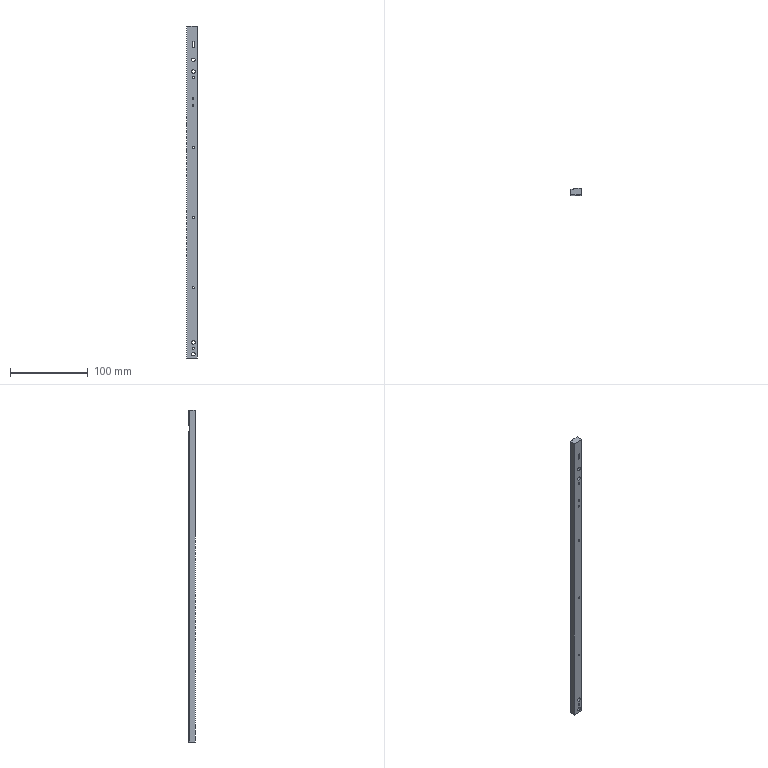Part | STEP file | 11-FG-B01111 | 1 solid | 58 faces | box 13.5 x 8.4 x 426 mm | volume 45040 mm3 | cylinder 34 | plane 20 | cone 4 | commonest cylinder face diameters 2.5 x18 4.5 x8 8 x8